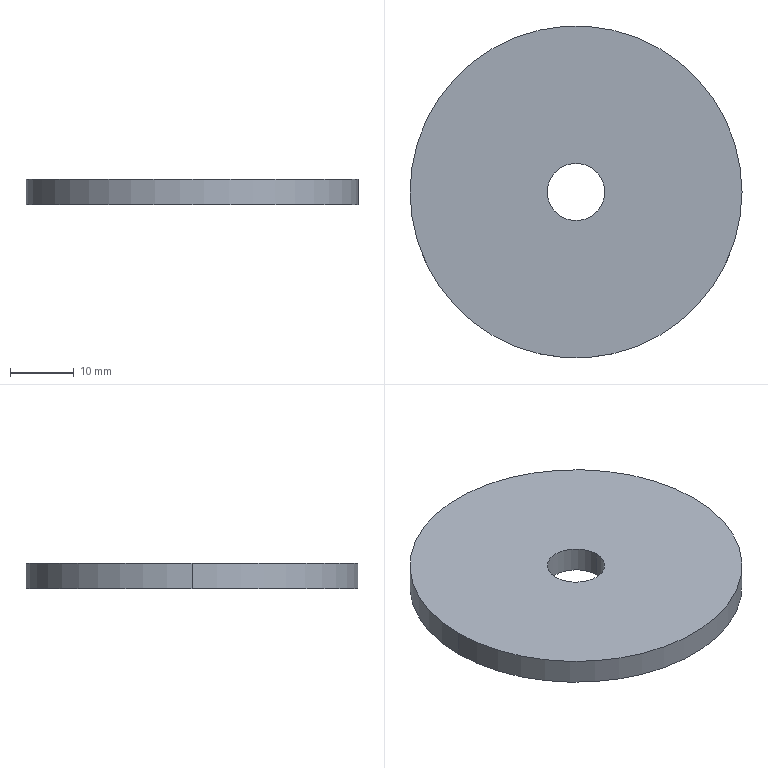Part | STEP file | limit plate_default | 1 solid | 6 faces | box 52 x 52 x 4 mm | volume 8240 mm3 | cylinder 4 | plane 2 | commonest cylinder face diameters 9 x2 52 x2
STEP:
#1=CARTESIAN_POINT('',(0.,0.,0.));
#2=DIRECTION('',(0.,0.,1.));
#3=DIRECTION('',(1.,0.,0.));
#4=AXIS2_PLACEMENT_3D('',#1,#2,#3);
#5=CARTESIAN_POINT('',(-4.5,0.,4.));
#6=VERTEX_POINT('',#5);
#7=CARTESIAN_POINT('',(-4.5,0.,0.));
#8=VERTEX_POINT('',#7);
#9=CARTESIAN_POINT('',(-4.5,0.,4.));
#10=DIRECTION('',(0.,0.,-1.));
#11=VECTOR('',#10,1.);
#12=LINE('',#9,#11);
#13=CARTESIAN_POINT('',(0.,0.,4.));
#14=DIRECTION('',(0.,0.,-1.));
#15=DIRECTION('',(-1.,0.,0.));
#16=AXIS2_PLACEMENT_3D('',#13,#14,#15);
#17=CYLINDRICAL_SURFACE('',#16,4.5);
#18=CARTESIAN_POINT('',(6.283,0.));
#19=DIRECTION('',(0.,1.));
#20=VECTOR('',#19,1.);
#21=LINE('',#18,#20);
#22=(GEOMETRIC_REPRESENTATION_CONTEXT(2)PARAMETRIC_REPRESENTATION_CONTEXT()REPRESENTATION_CONTEXT('',''));
#23=DEFINITIONAL_REPRESENTATION('',(#21),#22);
#24=PCURVE('',#17,#23);
#25=CARTESIAN_POINT('',(0.,0.,4.));
#26=DIRECTION('',(0.,0.,-1.));
#27=DIRECTION('',(-1.,0.,0.));
#28=AXIS2_PLACEMENT_3D('',#25,#26,#27);
#29=CYLINDRICAL_SURFACE('',#28,4.5);
#30=CARTESIAN_POINT('',(0.,0.));
#31=DIRECTION('',(0.,1.));
#32=VECTOR('',#31,1.);
#33=LINE('',#30,#32);
#34=(GEOMETRIC_REPRESENTATION_CONTEXT(2)PARAMETRIC_REPRESENTATION_CONTEXT()REPRESENTATION_CONTEXT('',''));
#35=DEFINITIONAL_REPRESENTATION('',(#33),#34);
#36=PCURVE('',#29,#35);
#37=SURFACE_CURVE('',#12,(#24,#36),.PCURVE_S1.);
#38=EDGE_CURVE('',#6,#8,#37,.T.);
#39=ORIENTED_EDGE('',*,*,#38,.T.);
#40=CARTESIAN_POINT('',(4.5,0.,0.));
#41=VERTEX_POINT('',#40);
#42=CARTESIAN_POINT('',(0.,0.,0.));
#43=DIRECTION('',(0.,0.,1.));
#44=DIRECTION('',(1.,0.,0.));
#45=AXIS2_PLACEMENT_3D('',#42,#43,#44);
#46=CIRCLE('',#45,4.5);
#47=CARTESIAN_POINT('',(9.425,4.));
#48=DIRECTION('',(-1.,0.));
#49=VECTOR('',#48,1.);
#50=LINE('',#47,#49);
#51=(GEOMETRIC_REPRESENTATION_CONTEXT(2)PARAMETRIC_REPRESENTATION_CONTEXT()REPRESENTATION_CONTEXT('',''));
#52=DEFINITIONAL_REPRESENTATION('',(#50),#51);
#53=PCURVE('',#17,#52);
#54=CARTESIAN_POINT('',(0.,0.,0.));
#55=DIRECTION('',(0.,0.,1.));
#56=DIRECTION('',(1.,0.,0.));
#57=AXIS2_PLACEMENT_3D('',#54,#55,#56);
#58=PLANE('',#57);
#59=CARTESIAN_POINT('',(0.,0.));
#60=DIRECTION('',(1.,0.));
#61=AXIS2_PLACEMENT_2D('',#59,#60);
#62=CIRCLE('',#61,4.5);
#63=(GEOMETRIC_REPRESENTATION_CONTEXT(2)PARAMETRIC_REPRESENTATION_CONTEXT()REPRESENTATION_CONTEXT('',''));
#64=DEFINITIONAL_REPRESENTATION('',(#62),#63);
#65=PCURVE('',#58,#64);
#66=SURFACE_CURVE('',#46,(#53,#65),.PCURVE_S1.);
#67=EDGE_CURVE('',#8,#41,#66,.T.);
#68=ORIENTED_EDGE('',*,*,#67,.T.);
#69=CARTESIAN_POINT('',(4.5,0.,4.));
#70=VERTEX_POINT('',#69);
#71=CARTESIAN_POINT('',(4.5,0.,4.));
#72=DIRECTION('',(0.,0.,-1.));
#73=VECTOR('',#72,1.);
#74=LINE('',#71,#73);
#75=CARTESIAN_POINT('',(3.142,0.));
#76=DIRECTION('',(0.,1.));
#77=VECTOR('',#76,1.);
#78=LINE('',#75,#77);
#79=(GEOMETRIC_REPRESENTATION_CONTEXT(2)PARAMETRIC_REPRESENTATION_CONTEXT()REPRESENTATION_CONTEXT('',''));
#80=DEFINITIONAL_REPRESENTATION('',(#78),#79);
#81=PCURVE('',#17,#80);
#82=CARTESIAN_POINT('',(3.142,0.));
#83=DIRECTION('',(0.,1.));
#84=VECTOR('',#83,1.);
#85=LINE('',#82,#84);
#86=(GEOMETRIC_REPRESENTATION_CONTEXT(2)PARAMETRIC_REPRESENTATION_CONTEXT()REPRESENTATION_CONTEXT('',''));
#87=DEFINITIONAL_REPRESENTATION('',(#85),#86);
#88=PCURVE('',#29,#87);
#89=SURFACE_CURVE('',#74,(#81,#88),.PCURVE_S1.);
#90=EDGE_CURVE('',#70,#41,#89,.T.);
#91=ORIENTED_EDGE('',*,*,#90,.F.);
#92=CARTESIAN_POINT('',(0.,0.,4.));
#93=DIRECTION('',(0.,0.,1.));
#94=DIRECTION('',(1.,0.,0.));
#95=AXIS2_PLACEMENT_3D('',#92,#93,#94);
#96=CIRCLE('',#95,4.5);
#97=CARTESIAN_POINT('',(9.425,0.));
#98=DIRECTION('',(-1.,0.));
#99=VECTOR('',#98,1.);
#100=LINE('',#97,#99);
#101=(GEOMETRIC_REPRESENTATION_CONTEXT(2)PARAMETRIC_REPRESENTATION_CONTEXT()REPRESENTATION_CONTEXT('',''));
#102=DEFINITIONAL_REPRESENTATION('',(#100),#101);
#103=PCURVE('',#17,#102);
#104=CARTESIAN_POINT('',(0.,0.,4.));
#105=DIRECTION('',(0.,0.,1.));
#106=DIRECTION('',(1.,0.,0.));
#107=AXIS2_PLACEMENT_3D('',#104,#105,#106);
#108=PLANE('',#107);
#109=CARTESIAN_POINT('',(0.,0.));
#110=DIRECTION('',(1.,0.));
#111=AXIS2_PLACEMENT_2D('',#109,#110);
#112=CIRCLE('',#111,4.5);
#113=(GEOMETRIC_REPRESENTATION_CONTEXT(2)PARAMETRIC_REPRESENTATION_CONTEXT()REPRESENTATION_CONTEXT('',''));
#114=DEFINITIONAL_REPRESENTATION('',(#112),#113);
#115=PCURVE('',#108,#114);
#116=SURFACE_CURVE('',#96,(#103,#115),.PCURVE_S1.);
#117=EDGE_CURVE('',#6,#70,#116,.T.);
#118=ORIENTED_EDGE('',*,*,#117,.F.);
#119=EDGE_LOOP('',(#39,#68,#91,#118));
#120=FACE_BOUND('',#119,.F.);
#121=ADVANCED_FACE('',(#120),#17,.F.);
#122=CARTESIAN_POINT('',(26.,0.,4.));
#123=VERTEX_POINT('',#122);
#124=CARTESIAN_POINT('',(-26.,0.,4.));
#125=VERTEX_POINT('',#124);
#126=CARTESIAN_POINT('',(0.,0.,4.));
#127=DIRECTION('',(0.,0.,1.));
#128=DIRECTION('',(1.,0.,0.));
#129=AXIS2_PLACEMENT_3D('',#126,#127,#128);
#130=CIRCLE('',#129,26.);
#131=CARTESIAN_POINT('',(0.,0.,4.));
#132=DIRECTION('',(0.,0.,-1.));
#133=DIRECTION('',(-1.,0.,0.));
#134=AXIS2_PLACEMENT_3D('',#131,#132,#133);
#135=CYLINDRICAL_SURFACE('',#134,26.);
#136=CARTESIAN_POINT('',(3.142,0.));
#137=DIRECTION('',(-1.,0.));
#138=VECTOR('',#137,1.);
#139=LINE('',#136,#138);
#140=(GEOMETRIC_REPRESENTATION_CONTEXT(2)PARAMETRIC_REPRESENTATION_CONTEXT()REPRESENTATION_CONTEXT('',''));
#141=DEFINITIONAL_REPRESENTATION('',(#139),#140);
#142=PCURVE('',#135,#141);
#143=CARTESIAN_POINT('',(0.,0.));
#144=DIRECTION('',(1.,0.));
#145=AXIS2_PLACEMENT_2D('',#143,#144);
#146=CIRCLE('',#145,26.);
#147=(GEOMETRIC_REPRESENTATION_CONTEXT(2)PARAMETRIC_REPRESENTATION_CONTEXT()REPRESENTATION_CONTEXT('',''));
#148=DEFINITIONAL_REPRESENTATION('',(#146),#147);
#149=PCURVE('',#108,#148);
#150=SURFACE_CURVE('',#130,(#142,#149),.PCURVE_S1.);
#151=EDGE_CURVE('',#123,#125,#150,.T.);
#152=ORIENTED_EDGE('',*,*,#151,.F.);
#153=CARTESIAN_POINT('',(26.,0.,0.));
#154=VERTEX_POINT('',#153);
#155=CARTESIAN_POINT('',(26.,0.,4.));
#156=DIRECTION('',(0.,0.,-1.));
#157=VECTOR('',#156,1.);
#158=LINE('',#155,#157);
#159=CARTESIAN_POINT('',(3.142,0.));
#160=DIRECTION('',(0.,1.));
#161=VECTOR('',#160,1.);
#162=LINE('',#159,#161);
#163=(GEOMETRIC_REPRESENTATION_CONTEXT(2)PARAMETRIC_REPRESENTATION_CONTEXT()REPRESENTATION_CONTEXT('',''));
#164=DEFINITIONAL_REPRESENTATION('',(#162),#163);
#165=PCURVE('',#135,#164);
#166=CARTESIAN_POINT('',(0.,0.,4.));
#167=DIRECTION('',(0.,0.,-1.));
#168=DIRECTION('',(-1.,0.,0.));
#169=AXIS2_PLACEMENT_3D('',#166,#167,#168);
#170=CYLINDRICAL_SURFACE('',#169,26.);
#171=CARTESIAN_POINT('',(3.142,0.));
#172=DIRECTION('',(0.,1.));
#173=VECTOR('',#172,1.);
#174=LINE('',#171,#173);
#175=(GEOMETRIC_REPRESENTATION_CONTEXT(2)PARAMETRIC_REPRESENTATION_CONTEXT()REPRESENTATION_CONTEXT('',''));
#176=DEFINITIONAL_REPRESENTATION('',(#174),#175);
#177=PCURVE('',#170,#176);
#178=SURFACE_CURVE('',#158,(#165,#177),.PCURVE_S1.);
#179=EDGE_CURVE('',#123,#154,#178,.T.);
#180=ORIENTED_EDGE('',*,*,#179,.T.);
#181=CARTESIAN_POINT('',(-26.,0.,0.));
#182=VERTEX_POINT('',#181);
#183=CARTESIAN_POINT('',(0.,0.,0.));
#184=DIRECTION('',(0.,0.,1.));
#185=DIRECTION('',(1.,0.,0.));
#186=AXIS2_PLACEMENT_3D('',#183,#184,#185);
#187=CIRCLE('',#186,26.);
#188=CARTESIAN_POINT('',(3.142,4.));
#189=DIRECTION('',(-1.,0.));
#190=VECTOR('',#189,1.);
#191=LINE('',#188,#190);
#192=(GEOMETRIC_REPRESENTATION_CONTEXT(2)PARAMETRIC_REPRESENTATION_CONTEXT()REPRESENTATION_CONTEXT('',''));
#193=DEFINITIONAL_REPRESENTATION('',(#191),#192);
#194=PCURVE('',#135,#193);
#195=CARTESIAN_POINT('',(0.,0.));
#196=DIRECTION('',(1.,0.));
#197=AXIS2_PLACEMENT_2D('',#195,#196);
#198=CIRCLE('',#197,26.);
#199=(GEOMETRIC_REPRESENTATION_CONTEXT(2)PARAMETRIC_REPRESENTATION_CONTEXT()REPRESENTATION_CONTEXT('',''));
#200=DEFINITIONAL_REPRESENTATION('',(#198),#199);
#201=PCURVE('',#58,#200);
#202=SURFACE_CURVE('',#187,(#194,#201),.PCURVE_S1.);
#203=EDGE_CURVE('',#154,#182,#202,.T.);
#204=ORIENTED_EDGE('',*,*,#203,.T.);
#205=CARTESIAN_POINT('',(-26.,0.,4.));
#206=DIRECTION('',(0.,0.,-1.));
#207=VECTOR('',#206,1.);
#208=LINE('',#205,#207);
#209=CARTESIAN_POINT('',(0.,0.));
#210=DIRECTION('',(0.,1.));
#211=VECTOR('',#210,1.);
#212=LINE('',#209,#211);
#213=(GEOMETRIC_REPRESENTATION_CONTEXT(2)PARAMETRIC_REPRESENTATION_CONTEXT()REPRESENTATION_CONTEXT('',''));
#214=DEFINITIONAL_REPRESENTATION('',(#212),#213);
#215=PCURVE('',#135,#214);
#216=CARTESIAN_POINT('',(6.283,0.));
#217=DIRECTION('',(0.,1.));
#218=VECTOR('',#217,1.);
#219=LINE('',#216,#218);
#220=(GEOMETRIC_REPRESENTATION_CONTEXT(2)PARAMETRIC_REPRESENTATION_CONTEXT()REPRESENTATION_CONTEXT('',''));
#221=DEFINITIONAL_REPRESENTATION('',(#219),#220);
#222=PCURVE('',#170,#221);
#223=SURFACE_CURVE('',#208,(#215,#222),.PCURVE_S1.);
#224=EDGE_CURVE('',#125,#182,#223,.T.);
#225=ORIENTED_EDGE('',*,*,#224,.F.);
#226=EDGE_LOOP('',(#152,#180,#204,#225));
#227=FACE_BOUND('',#226,.T.);
#228=ADVANCED_FACE('',(#227),#135,.T.);
#229=CARTESIAN_POINT('',(0.,0.,4.));
#230=DIRECTION('',(0.,0.,1.));
#231=DIRECTION('',(1.,0.,0.));
#232=AXIS2_PLACEMENT_3D('',#229,#230,#231);
#233=CIRCLE('',#232,26.);
#234=CARTESIAN_POINT('',(0.,0.));
#235=DIRECTION('',(1.,0.));
#236=AXIS2_PLACEMENT_2D('',#234,#235);
#237=CIRCLE('',#236,26.);
#238=(GEOMETRIC_REPRESENTATION_CONTEXT(2)PARAMETRIC_REPRESENTATION_CONTEXT()REPRESENTATION_CONTEXT('',''));
#239=DEFINITIONAL_REPRESENTATION('',(#237),#238);
#240=PCURVE('',#108,#239);
#241=CARTESIAN_POINT('',(9.425,0.));
#242=DIRECTION('',(-1.,0.));
#243=VECTOR('',#242,1.);
#244=LINE('',#241,#243);
#245=(GEOMETRIC_REPRESENTATION_CONTEXT(2)PARAMETRIC_REPRESENTATION_CONTEXT()REPRESENTATION_CONTEXT('',''));
#246=DEFINITIONAL_REPRESENTATION('',(#244),#245);
#247=PCURVE('',#170,#246);
#248=SURFACE_CURVE('',#233,(#240,#247),.PCURVE_S1.);
#249=EDGE_CURVE('',#125,#123,#248,.T.);
#250=ORIENTED_EDGE('',*,*,#249,.T.);
#251=ORIENTED_EDGE('',*,*,#151,.T.);
#252=EDGE_LOOP('',(#250,#251));
#253=FACE_BOUND('',#252,.T.);
#254=ORIENTED_EDGE('',*,*,#117,.F.);
#255=CARTESIAN_POINT('',(0.,0.,4.));
#256=DIRECTION('',(0.,0.,1.));
#257=DIRECTION('',(1.,0.,0.));
#258=AXIS2_PLACEMENT_3D('',#255,#256,#257);
#259=CIRCLE('',#258,4.5);
#260=CARTESIAN_POINT('',(0.,0.));
#261=DIRECTION('',(1.,0.));
#262=AXIS2_PLACEMENT_2D('',#260,#261);
#263=CIRCLE('',#262,4.5);
#264=(GEOMETRIC_REPRESENTATION_CONTEXT(2)PARAMETRIC_REPRESENTATION_CONTEXT()REPRESENTATION_CONTEXT('',''));
#265=DEFINITIONAL_REPRESENTATION('',(#263),#264);
#266=PCURVE('',#108,#265);
#267=CARTESIAN_POINT('',(3.142,0.));
#268=DIRECTION('',(-1.,0.));
#269=VECTOR('',#268,1.);
#270=LINE('',#267,#269);
#271=(GEOMETRIC_REPRESENTATION_CONTEXT(2)PARAMETRIC_REPRESENTATION_CONTEXT()REPRESENTATION_CONTEXT('',''));
#272=DEFINITIONAL_REPRESENTATION('',(#270),#271);
#273=PCURVE('',#29,#272);
#274=SURFACE_CURVE('',#259,(#266,#273),.PCURVE_S1.);
#275=EDGE_CURVE('',#70,#6,#274,.T.);
#276=ORIENTED_EDGE('',*,*,#275,.F.);
#277=EDGE_LOOP('',(#254,#276));
#278=FACE_BOUND('',#277,.T.);
#279=ADVANCED_FACE('',(#253,#278),#108,.T.);
#280=CARTESIAN_POINT('',(0.,0.,0.));
#281=DIRECTION('',(0.,0.,1.));
#282=DIRECTION('',(1.,0.,0.));
#283=AXIS2_PLACEMENT_3D('',#280,#281,#282);
#284=CIRCLE('',#283,26.);
#285=CARTESIAN_POINT('',(0.,0.));
#286=DIRECTION('',(1.,0.));
#287=AXIS2_PLACEMENT_2D('',#285,#286);
#288=CIRCLE('',#287,26.);
#289=(GEOMETRIC_REPRESENTATION_CONTEXT(2)PARAMETRIC_REPRESENTATION_CONTEXT()REPRESENTATION_CONTEXT('',''));
#290=DEFINITIONAL_REPRESENTATION('',(#288),#289);
#291=PCURVE('',#58,#290);
#292=CARTESIAN_POINT('',(9.425,4.));
#293=DIRECTION('',(-1.,0.));
#294=VECTOR('',#293,1.);
#295=LINE('',#292,#294);
#296=(GEOMETRIC_REPRESENTATION_CONTEXT(2)PARAMETRIC_REPRESENTATION_CONTEXT()REPRESENTATION_CONTEXT('',''));
#297=DEFINITIONAL_REPRESENTATION('',(#295),#296);
#298=PCURVE('',#170,#297);
#299=SURFACE_CURVE('',#284,(#291,#298),.PCURVE_S1.);
#300=EDGE_CURVE('',#182,#154,#299,.T.);
#301=ORIENTED_EDGE('',*,*,#300,.F.);
#302=ORIENTED_EDGE('',*,*,#203,.F.);
#303=EDGE_LOOP('',(#301,#302));
#304=FACE_BOUND('',#303,.T.);
#305=ORIENTED_EDGE('',*,*,#67,.T.);
#306=CARTESIAN_POINT('',(0.,0.,0.));
#307=DIRECTION('',(0.,0.,1.));
#308=DIRECTION('',(1.,0.,0.));
#309=AXIS2_PLACEMENT_3D('',#306,#307,#308);
#310=CIRCLE('',#309,4.5);
#311=CARTESIAN_POINT('',(0.,0.));
#312=DIRECTION('',(1.,0.));
#313=AXIS2_PLACEMENT_2D('',#311,#312);
#314=CIRCLE('',#313,4.5);
#315=(GEOMETRIC_REPRESENTATION_CONTEXT(2)PARAMETRIC_REPRESENTATION_CONTEXT()REPRESENTATION_CONTEXT('',''));
#316=DEFINITIONAL_REPRESENTATION('',(#314),#315);
#317=PCURVE('',#58,#316);
#318=CARTESIAN_POINT('',(3.142,4.));
#319=DIRECTION('',(-1.,0.));
#320=VECTOR('',#319,1.);
#321=LINE('',#318,#320);
#322=(GEOMETRIC_REPRESENTATION_CONTEXT(2)PARAMETRIC_REPRESENTATION_CONTEXT()REPRESENTATION_CONTEXT('',''));
#323=DEFINITIONAL_REPRESENTATION('',(#321),#322);
#324=PCURVE('',#29,#323);
#325=SURFACE_CURVE('',#310,(#317,#324),.PCURVE_S1.);
#326=EDGE_CURVE('',#41,#8,#325,.T.);
#327=ORIENTED_EDGE('',*,*,#326,.T.);
#328=EDGE_LOOP('',(#305,#327));
#329=FACE_BOUND('',#328,.T.);
#330=ADVANCED_FACE('',(#304,#329),#58,.F.);
#331=ORIENTED_EDGE('',*,*,#179,.F.);
#332=ORIENTED_EDGE('',*,*,#249,.F.);
#333=ORIENTED_EDGE('',*,*,#224,.T.);
#334=ORIENTED_EDGE('',*,*,#300,.T.);
#335=EDGE_LOOP('',(#331,#332,#333,#334));
#336=FACE_BOUND('',#335,.T.);
#337=ADVANCED_FACE('',(#336),#170,.T.);
#338=ORIENTED_EDGE('',*,*,#326,.T.);
#339=ORIENTED_EDGE('',*,*,#38,.F.);
#340=ORIENTED_EDGE('',*,*,#275,.F.);
#341=ORIENTED_EDGE('',*,*,#90,.T.);
#342=EDGE_LOOP('',(#338,#339,#340,#341));
#343=FACE_BOUND('',#342,.F.);
#344=ADVANCED_FACE('',(#343),#29,.F.);
#345=CLOSED_SHELL('',(#121,#228,#279,#330,#337,#344));
#346=MANIFOLD_SOLID_BREP('',#345);
#347=(LENGTH_UNIT()NAMED_UNIT(*)SI_UNIT(.MILLI.,.METRE.));
#348=UNCERTAINTY_MEASURE_WITH_UNIT(LENGTH_MEASURE(0.0000001),#347,'','');
#349=(NAMED_UNIT(*)PLANE_ANGLE_UNIT()SI_UNIT($,.RADIAN.));
#350=(NAMED_UNIT(*)SI_UNIT($,.STERADIAN.)SOLID_ANGLE_UNIT());
#351=(GEOMETRIC_REPRESENTATION_CONTEXT(3)GLOBAL_UNCERTAINTY_ASSIGNED_CONTEXT((#348))GLOBAL_UNIT_ASSIGNED_CONTEXT((#347,#349,#350))REPRESENTATION_CONTEXT('',''));
#352=ADVANCED_BREP_SHAPE_REPRESENTATION('',(#4,#346),#351);